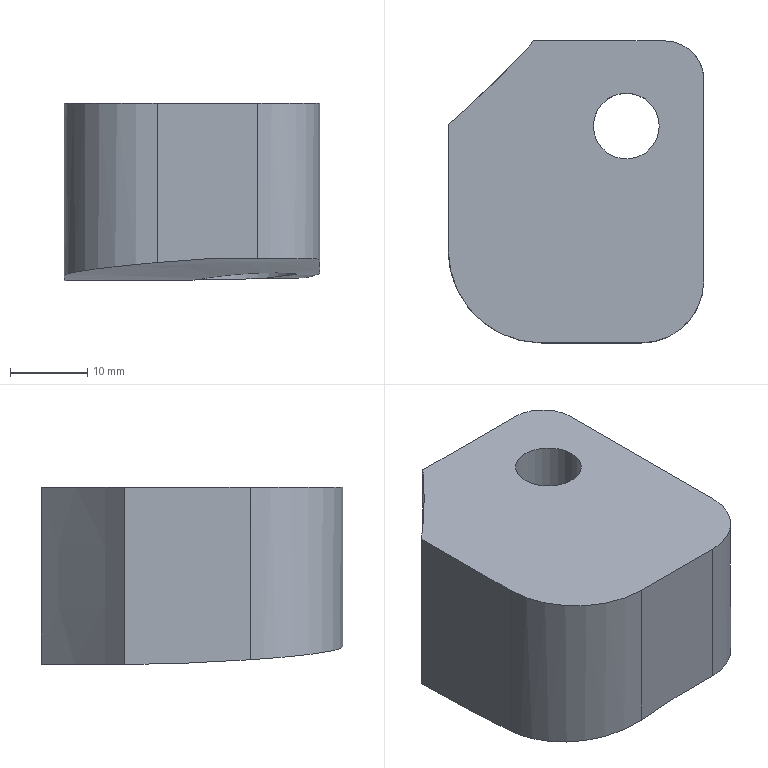Part | STEP file | gslz 2016.10.28-10_id2138_x_t | 1 solid | 13 faces | box 33 x 39 x 22.871 mm | volume 23188 mm3 | plane 6 | cylinder 5 | spline 1 | other 1 | commonest cylinder face diameters 8.5 x1 10 x1 14 x1 16 x1 24 x1